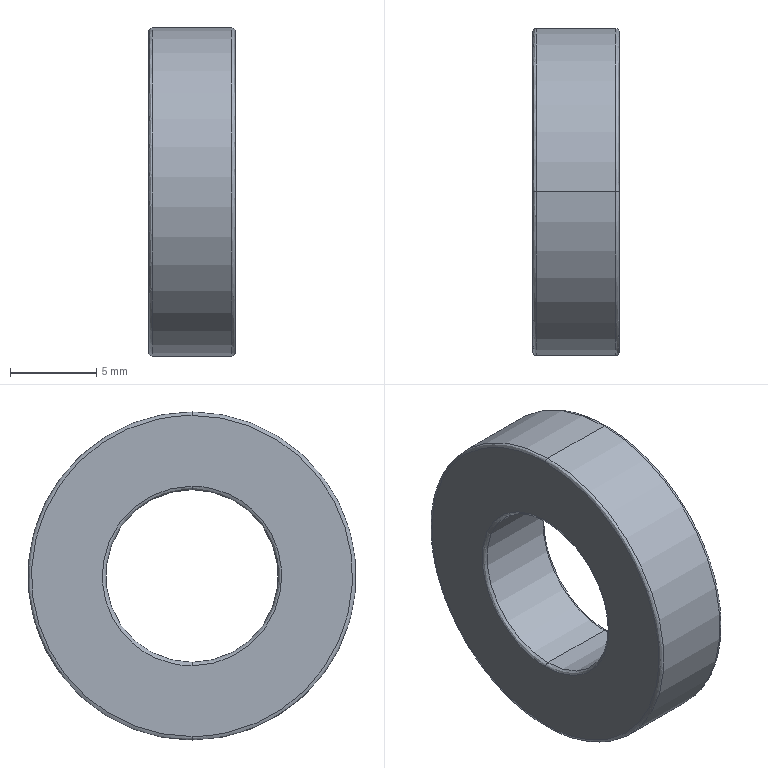Part | STEP file | Bearing SB6800ZZ | 1 solid | 14 faces | box 5 x 19 x 19 mm | volume 1023 mm3 | spline 8 | cylinder 4 | plane 2 | commonest cylinder face diameters 10 x2 19 x2